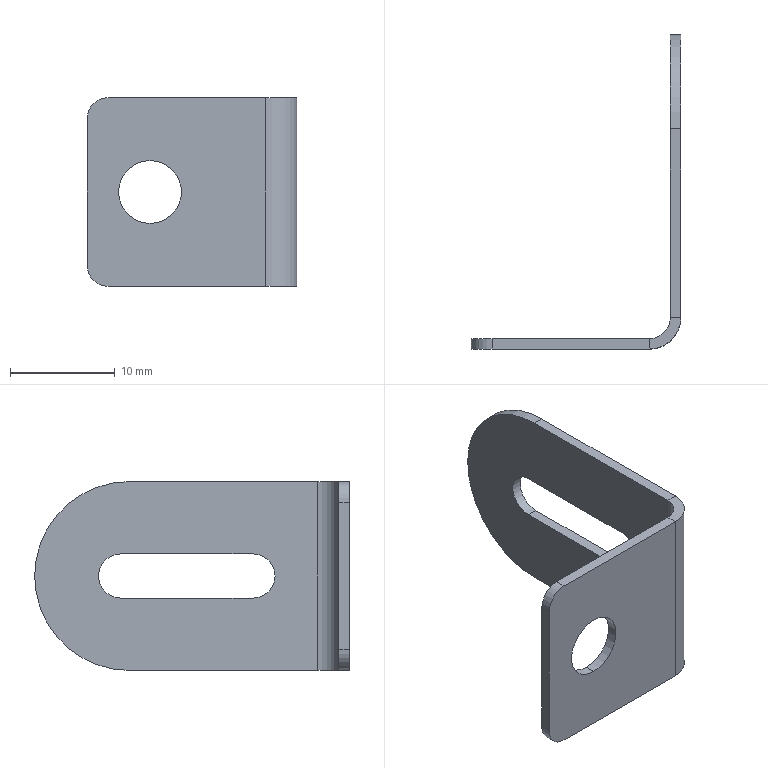Part | SolidWorks | features Fillet 2, ICE 2, EdgeFlange 1, FlatPattern 1, SMBaseFlange 1, SheetMetal 1 | 1 solid | 24 faces | box 20 x 30 x 18 mm | volume 730.964 mm3 | plane 13 | cylinder 11 | commonest cylinder face diameters 4 x3 4.2 x3 6 x3 18 x2
STEP:
#1=CARTESIAN_POINT('',(10.,8.173,2.1));
#2=VERTEX_POINT('',#1);
#3=CARTESIAN_POINT('',(10.,6.073,0.));
#4=VERTEX_POINT('',#3);
#5=CARTESIAN_POINT('',(10.,8.173,0.));
#6=DIRECTION('',(1.,0.,0.));
#7=DIRECTION('',(0.,1.,0.));
#8=AXIS2_PLACEMENT_3D('',#5,#6,#7);
#9=CIRCLE('',#8,2.1);
#10=EDGE_CURVE('',#2,#4,#9,.T.);
#11=ORIENTED_EDGE('',*,*,#10,.T.);
#12=CARTESIAN_POINT('',(9.,6.073,0.));
#13=VERTEX_POINT('',#12);
#14=CARTESIAN_POINT('',(19.,6.073,0.));
#15=DIRECTION('',(-1.,0.,0.));
#16=VECTOR('',#15,1000.);
#17=LINE('',#14,#16);
#18=EDGE_CURVE('',#4,#13,#17,.T.);
#19=ORIENTED_EDGE('',*,*,#18,.T.);
#20=CARTESIAN_POINT('',(9.,8.173,2.1));
#21=VERTEX_POINT('',#20);
#22=CARTESIAN_POINT('',(9.,8.173,0.));
#23=DIRECTION('',(-1.,0.,0.));
#24=DIRECTION('',(0.,-1.,0.));
#25=AXIS2_PLACEMENT_3D('',#22,#23,#24);
#26=CIRCLE('',#25,2.1);
#27=EDGE_CURVE('',#13,#21,#26,.T.);
#28=ORIENTED_EDGE('',*,*,#27,.T.);
#29=CARTESIAN_POINT('',(19.,8.173,2.1));
#30=DIRECTION('',(-1.,0.,0.));
#31=VECTOR('',#30,1000.);
#32=LINE('',#29,#31);
#33=EDGE_CURVE('',#2,#21,#32,.T.);
#34=ORIENTED_EDGE('',*,*,#33,.F.);
#35=EDGE_LOOP('',(#11,#19,#28,#34));
#36=FACE_OUTER_BOUND('',#35,.T.);
#37=CARTESIAN_POINT('',(19.,8.173,0.));
#38=DIRECTION('',(-1.,0.,0.));
#39=DIRECTION('',(0.,-1.,0.));
#40=AXIS2_PLACEMENT_3D('',#37,#38,#39);
#41=CYLINDRICAL_SURFACE('',#40,2.1);
#42=ADVANCED_FACE('',(#36),#41,.F.);
#43=CARTESIAN_POINT('',(-4.,-1.,-3.));
#44=VERTEX_POINT('',#43);
#45=CARTESIAN_POINT('',(-4.,-1.,3.));
#46=VERTEX_POINT('',#45);
#47=CARTESIAN_POINT('',(-4.,-1.,0.));
#48=DIRECTION('',(0.,1.,0.));
#49=DIRECTION('',(0.,0.,1.));
#50=AXIS2_PLACEMENT_3D('',#47,#48,#49);
#51=CIRCLE('',#50,3.);
#52=EDGE_CURVE('',#44,#46,#51,.T.);
#53=ORIENTED_EDGE('',*,*,#52,.F.);
#54=CARTESIAN_POINT('',(-4.,0.,-3.));
#55=VERTEX_POINT('',#54);
#56=CARTESIAN_POINT('',(-4.,-10.,-3.));
#57=DIRECTION('',(0.,1.,0.));
#58=VECTOR('',#57,1000.);
#59=LINE('',#56,#58);
#60=EDGE_CURVE('',#44,#55,#59,.T.);
#61=ORIENTED_EDGE('',*,*,#60,.T.);
#62=CARTESIAN_POINT('',(-4.,0.,3.));
#63=VERTEX_POINT('',#62);
#64=CARTESIAN_POINT('',(-4.,0.,0.));
#65=DIRECTION('',(0.,1.,0.));
#66=DIRECTION('',(0.,0.,1.));
#67=AXIS2_PLACEMENT_3D('',#64,#65,#66);
#68=CIRCLE('',#67,3.);
#69=EDGE_CURVE('',#55,#63,#68,.T.);
#70=ORIENTED_EDGE('',*,*,#69,.T.);
#71=CARTESIAN_POINT('',(-4.,-10.,3.));
#72=DIRECTION('',(0.,1.,0.));
#73=VECTOR('',#72,1000.);
#74=LINE('',#71,#73);
#75=EDGE_CURVE('',#46,#63,#74,.T.);
#76=ORIENTED_EDGE('',*,*,#75,.F.);
#77=EDGE_LOOP('',(#53,#61,#70,#76));
#78=FACE_OUTER_BOUND('',#77,.T.);
#79=CARTESIAN_POINT('',(-4.,-10.,0.));
#80=DIRECTION('',(0.,1.,0.));
#81=DIRECTION('',(0.,0.,1.));
#82=AXIS2_PLACEMENT_3D('',#79,#80,#81);
#83=CYLINDRICAL_SURFACE('',#82,3.);
#84=ADVANCED_FACE('',(#78),#83,.F.);
#85=CARTESIAN_POINT('',(7.,-1.,-9.));
#86=VERTEX_POINT('',#85);
#87=CARTESIAN_POINT('',(-8.,-1.,-9.));
#88=VERTEX_POINT('',#87);
#89=CARTESIAN_POINT('',(-10.,-1.,-9.));
#90=DIRECTION('',(-1.,0.,0.));
#91=VECTOR('',#90,1000.);
#92=LINE('',#89,#91);
#93=EDGE_CURVE('',#86,#88,#92,.T.);
#94=ORIENTED_EDGE('',*,*,#93,.T.);
#95=CARTESIAN_POINT('',(-8.,0.,-9.));
#96=VERTEX_POINT('',#95);
#97=CARTESIAN_POINT('',(-8.,-1.,-9.));
#98=DIRECTION('',(0.,1.,0.));
#99=VECTOR('',#98,1000.);
#100=LINE('',#97,#99);
#101=EDGE_CURVE('',#88,#96,#100,.T.);
#102=ORIENTED_EDGE('',*,*,#101,.T.);
#103=CARTESIAN_POINT('',(7.,0.,-9.));
#104=VERTEX_POINT('',#103);
#105=CARTESIAN_POINT('',(-10.,0.,-9.));
#106=DIRECTION('',(-1.,0.,0.));
#107=VECTOR('',#106,1000.);
#108=LINE('',#105,#107);
#109=EDGE_CURVE('',#104,#96,#108,.T.);
#110=ORIENTED_EDGE('',*,*,#109,.F.);
#111=CARTESIAN_POINT('',(7.,0.,-9.));
#112=DIRECTION('',(0.,-1.,0.));
#113=VECTOR('',#112,1000.);
#114=LINE('',#111,#113);
#115=EDGE_CURVE('',#104,#86,#114,.T.);
#116=ORIENTED_EDGE('',*,*,#115,.T.);
#117=EDGE_LOOP('',(#94,#102,#110,#116));
#118=FACE_OUTER_BOUND('',#117,.T.);
#119=CARTESIAN_POINT('',(-10.,-1.,-9.));
#120=DIRECTION('',(0.,0.,-1.));
#121=DIRECTION('',(-1.,0.,0.));
#122=AXIS2_PLACEMENT_3D('',#119,#120,#121);
#123=PLANE('',#122);
#124=ADVANCED_FACE('',(#118),#123,.T.);
#125=CARTESIAN_POINT('',(-4.,-1.,0.));
#126=DIRECTION('',(0.,1.,0.));
#127=DIRECTION('',(0.,0.,1.));
#128=AXIS2_PLACEMENT_3D('',#125,#126,#127);
#129=CIRCLE('',#128,3.);
#130=EDGE_CURVE('',#46,#44,#129,.T.);
#131=ORIENTED_EDGE('',*,*,#130,.T.);
#132=ORIENTED_EDGE('',*,*,#52,.T.);
#133=EDGE_LOOP('',(#131,#132));
#134=FACE_BOUND('',#133,.T.);
#135=CARTESIAN_POINT('',(-10.,-1.,-7.));
#136=VERTEX_POINT('',#135);
#137=CARTESIAN_POINT('',(-10.,-1.,7.));
#138=VERTEX_POINT('',#137);
#139=CARTESIAN_POINT('',(-10.,-1.,-9.));
#140=DIRECTION('',(0.,0.,1.));
#141=VECTOR('',#140,1000.);
#142=LINE('',#139,#141);
#143=EDGE_CURVE('',#136,#138,#142,.T.);
#144=ORIENTED_EDGE('',*,*,#143,.F.);
#145=CARTESIAN_POINT('',(-8.,-1.,-7.));
#146=DIRECTION('',(0.,-1.,0.));
#147=DIRECTION('',(0.,0.,1.));
#148=AXIS2_PLACEMENT_3D('',#145,#146,#147);
#149=CIRCLE('',#148,2.);
#150=EDGE_CURVE('',#136,#88,#149,.T.);
#151=ORIENTED_EDGE('',*,*,#150,.T.);
#152=ORIENTED_EDGE('',*,*,#93,.F.);
#153=CARTESIAN_POINT('',(7.,-1.,9.));
#154=VERTEX_POINT('',#153);
#155=CARTESIAN_POINT('',(7.,-1.,-9.));
#156=DIRECTION('',(0.,0.,1.));
#157=VECTOR('',#156,1000.);
#158=LINE('',#155,#157);
#159=EDGE_CURVE('',#86,#154,#158,.T.);
#160=ORIENTED_EDGE('',*,*,#159,.T.);
#161=CARTESIAN_POINT('',(-8.,-1.,9.));
#162=VERTEX_POINT('',#161);
#163=CARTESIAN_POINT('',(-10.,-1.,9.));
#164=DIRECTION('',(1.,0.,0.));
#165=VECTOR('',#164,1000.);
#166=LINE('',#163,#165);
#167=EDGE_CURVE('',#162,#154,#166,.T.);
#168=ORIENTED_EDGE('',*,*,#167,.F.);
#169=CARTESIAN_POINT('',(-8.,-1.,7.));
#170=DIRECTION('',(0.,-1.,0.));
#171=DIRECTION('',(0.,0.,1.));
#172=AXIS2_PLACEMENT_3D('',#169,#170,#171);
#173=CIRCLE('',#172,2.);
#174=EDGE_CURVE('',#162,#138,#173,.T.);
#175=ORIENTED_EDGE('',*,*,#174,.T.);
#176=EDGE_LOOP('',(#144,#151,#152,#160,#168,#175));
#177=FACE_OUTER_BOUND('',#176,.T.);
#178=CARTESIAN_POINT('',(0.,-1.,0.));
#179=DIRECTION('',(0.,1.,0.));
#180=DIRECTION('',(0.,0.,1.));
#181=AXIS2_PLACEMENT_3D('',#178,#179,#180);
#182=PLANE('',#181);
#183=ADVANCED_FACE('',(#134,#177),#182,.F.);
#184=CARTESIAN_POINT('',(-4.,0.,0.));
#185=DIRECTION('',(0.,1.,0.));
#186=DIRECTION('',(0.,0.,1.));
#187=AXIS2_PLACEMENT_3D('',#184,#185,#186);
#188=CIRCLE('',#187,3.);
#189=EDGE_CURVE('',#63,#55,#188,.T.);
#190=ORIENTED_EDGE('',*,*,#189,.F.);
#191=ORIENTED_EDGE('',*,*,#69,.F.);
#192=EDGE_LOOP('',(#190,#191));
#193=FACE_BOUND('',#192,.T.);
#194=ORIENTED_EDGE('',*,*,#109,.T.);
#195=CARTESIAN_POINT('',(-10.,0.,-7.));
#196=VERTEX_POINT('',#195);
#197=CARTESIAN_POINT('',(-8.,0.,-7.));
#198=DIRECTION('',(0.,1.,0.));
#199=DIRECTION('',(0.,0.,1.));
#200=AXIS2_PLACEMENT_3D('',#197,#198,#199);
#201=CIRCLE('',#200,2.);
#202=EDGE_CURVE('',#96,#196,#201,.T.);
#203=ORIENTED_EDGE('',*,*,#202,.T.);
#204=CARTESIAN_POINT('',(-10.,0.,7.));
#205=VERTEX_POINT('',#204);
#206=CARTESIAN_POINT('',(-10.,0.,-9.));
#207=DIRECTION('',(0.,0.,1.));
#208=VECTOR('',#207,1000.);
#209=LINE('',#206,#208);
#210=EDGE_CURVE('',#196,#205,#209,.T.);
#211=ORIENTED_EDGE('',*,*,#210,.T.);
#212=CARTESIAN_POINT('',(-8.,0.,9.));
#213=VERTEX_POINT('',#212);
#214=CARTESIAN_POINT('',(-8.,0.,7.));
#215=DIRECTION('',(0.,1.,0.));
#216=DIRECTION('',(0.,0.,1.));
#217=AXIS2_PLACEMENT_3D('',#214,#215,#216);
#218=CIRCLE('',#217,2.);
#219=EDGE_CURVE('',#205,#213,#218,.T.);
#220=ORIENTED_EDGE('',*,*,#219,.T.);
#221=CARTESIAN_POINT('',(7.,0.,9.));
#222=VERTEX_POINT('',#221);
#223=CARTESIAN_POINT('',(-10.,0.,9.));
#224=DIRECTION('',(1.,0.,0.));
#225=VECTOR('',#224,1000.);
#226=LINE('',#223,#225);
#227=EDGE_CURVE('',#213,#222,#226,.T.);
#228=ORIENTED_EDGE('',*,*,#227,.T.);
#229=CARTESIAN_POINT('',(7.,0.,-9.));
#230=DIRECTION('',(0.,0.,1.));
#231=VECTOR('',#230,1000.);
#232=LINE('',#229,#231);
#233=EDGE_CURVE('',#104,#222,#232,.T.);
#234=ORIENTED_EDGE('',*,*,#233,.F.);
#235=EDGE_LOOP('',(#194,#203,#211,#220,#228,#234));
#236=FACE_OUTER_BOUND('',#235,.T.);
#237=CARTESIAN_POINT('',(0.,0.,0.));
#238=DIRECTION('',(0.,1.,0.));
#239=DIRECTION('',(0.,0.,1.));
#240=AXIS2_PLACEMENT_3D('',#237,#238,#239);
#241=PLANE('',#240);
#242=ADVANCED_FACE('',(#193,#236),#241,.T.);
#243=ORIENTED_EDGE('',*,*,#227,.F.);
#244=CARTESIAN_POINT('',(-8.,-1.,9.));
#245=DIRECTION('',(0.,-1.,0.));
#246=VECTOR('',#245,1000.);
#247=LINE('',#244,#246);
#248=EDGE_CURVE('',#213,#162,#247,.T.);
#249=ORIENTED_EDGE('',*,*,#248,.T.);
#250=ORIENTED_EDGE('',*,*,#167,.T.);
#251=CARTESIAN_POINT('',(7.,0.,9.));
#252=DIRECTION('',(0.,-1.,0.));
#253=VECTOR('',#252,1000.);
#254=LINE('',#251,#253);
#255=EDGE_CURVE('',#222,#154,#254,.T.);
#256=ORIENTED_EDGE('',*,*,#255,.F.);
#257=EDGE_LOOP('',(#243,#249,#250,#256));
#258=FACE_OUTER_BOUND('',#257,.T.);
#259=CARTESIAN_POINT('',(-10.,-1.,9.));
#260=DIRECTION('',(0.,0.,1.));
#261=DIRECTION('',(1.,0.,0.));
#262=AXIS2_PLACEMENT_3D('',#259,#260,#261);
#263=PLANE('',#262);
#264=ADVANCED_FACE('',(#258),#263,.T.);
#265=ORIENTED_EDGE('',*,*,#210,.F.);
#266=CARTESIAN_POINT('',(-10.,-1.,-7.));
#267=DIRECTION('',(0.,-1.,0.));
#268=VECTOR('',#267,1000.);
#269=LINE('',#266,#268);
#270=EDGE_CURVE('',#196,#136,#269,.T.);
#271=ORIENTED_EDGE('',*,*,#270,.T.);
#272=ORIENTED_EDGE('',*,*,#143,.T.);
#273=CARTESIAN_POINT('',(-10.,-1.,7.));
#274=DIRECTION('',(0.,1.,0.));
#275=VECTOR('',#274,1000.);
#276=LINE('',#273,#275);
#277=EDGE_CURVE('',#138,#205,#276,.T.);
#278=ORIENTED_EDGE('',*,*,#277,.T.);
#279=EDGE_LOOP('',(#265,#271,#272,#278));
#280=FACE_OUTER_BOUND('',#279,.T.);
#281=CARTESIAN_POINT('',(-10.,-1.,-9.));
#282=DIRECTION('',(-1.,0.,0.));
#283=DIRECTION('',(0.,0.,1.));
#284=AXIS2_PLACEMENT_3D('',#281,#282,#283);
#285=PLANE('',#284);
#286=ADVANCED_FACE('',(#280),#285,.T.);
#287=CARTESIAN_POINT('',(9.,2.,9.));
#288=VERTEX_POINT('',#287);
#289=CARTESIAN_POINT('',(10.,2.,9.));
#290=VERTEX_POINT('',#289);
#291=CARTESIAN_POINT('',(10.,2.,9.));
#292=DIRECTION('',(1.,0.,0.));
#293=VECTOR('',#292,1000.);
#294=LINE('',#291,#293);
#295=EDGE_CURVE('',#288,#290,#294,.T.);
#296=ORIENTED_EDGE('',*,*,#295,.F.);
#297=CARTESIAN_POINT('',(7.,2.,9.));
#298=DIRECTION('',(0.,0.,1.));
#299=DIRECTION('',(-1.,0.,0.));
#300=AXIS2_PLACEMENT_3D('',#297,#298,#299);
#301=CIRCLE('',#300,2.);
#302=EDGE_CURVE('',#222,#288,#301,.T.);
#303=ORIENTED_EDGE('',*,*,#302,.F.);
#304=ORIENTED_EDGE('',*,*,#255,.T.);
#305=CARTESIAN_POINT('',(7.,2.,9.));
#306=DIRECTION('',(0.,0.,1.));
#307=DIRECTION('',(-1.,0.,0.));
#308=AXIS2_PLACEMENT_3D('',#305,#306,#307);
#309=CIRCLE('',#308,3.);
#310=EDGE_CURVE('',#154,#290,#309,.T.);
#311=ORIENTED_EDGE('',*,*,#310,.T.);
#312=EDGE_LOOP('',(#296,#303,#304,#311));
#313=FACE_OUTER_BOUND('',#312,.T.);
#314=CARTESIAN_POINT('',(7.,2.,9.));
#315=DIRECTION('',(0.,0.,1.));
#316=DIRECTION('',(1.,0.,0.));
#317=AXIS2_PLACEMENT_3D('',#314,#315,#316);
#318=PLANE('',#317);
#319=ADVANCED_FACE('',(#313),#318,.T.);
#320=CARTESIAN_POINT('',(9.,2.,-9.));
#321=VERTEX_POINT('',#320);
#322=CARTESIAN_POINT('',(7.,2.,-9.));
#323=DIRECTION('',(0.,0.,-1.));
#324=DIRECTION('',(-1.,0.,0.));
#325=AXIS2_PLACEMENT_3D('',#322,#323,#324);
#326=CIRCLE('',#325,2.);
#327=EDGE_CURVE('',#321,#104,#326,.T.);
#328=ORIENTED_EDGE('',*,*,#327,.F.);
#329=CARTESIAN_POINT('',(10.,2.,-9.));
#330=VERTEX_POINT('',#329);
#331=CARTESIAN_POINT('',(9.,2.,-9.));
#332=DIRECTION('',(1.,0.,0.));
#333=VECTOR('',#332,1000.);
#334=LINE('',#331,#333);
#335=EDGE_CURVE('',#321,#330,#334,.T.);
#336=ORIENTED_EDGE('',*,*,#335,.T.);
#337=CARTESIAN_POINT('',(7.,2.,-9.));
#338=DIRECTION('',(0.,0.,-1.));
#339=DIRECTION('',(-1.,0.,0.));
#340=AXIS2_PLACEMENT_3D('',#337,#338,#339);
#341=CIRCLE('',#340,3.);
#342=EDGE_CURVE('',#330,#86,#341,.T.);
#343=ORIENTED_EDGE('',*,*,#342,.T.);
#344=ORIENTED_EDGE('',*,*,#115,.F.);
#345=EDGE_LOOP('',(#328,#336,#343,#344));
#346=FACE_OUTER_BOUND('',#345,.T.);
#347=CARTESIAN_POINT('',(7.,2.,-9.));
#348=DIRECTION('',(0.,0.,1.));
#349=DIRECTION('',(1.,0.,0.));
#350=AXIS2_PLACEMENT_3D('',#347,#348,#349);
#351=PLANE('',#350);
#352=ADVANCED_FACE('',(#346),#351,.F.);
#353=ORIENTED_EDGE('',*,*,#159,.F.);
#354=ORIENTED_EDGE('',*,*,#342,.F.);
#355=CARTESIAN_POINT('',(10.,2.,0.));
#356=DIRECTION('',(0.,0.,-1.));
#357=VECTOR('',#356,1000.);
#358=LINE('',#355,#357);
#359=EDGE_CURVE('',#290,#330,#358,.T.);
#360=ORIENTED_EDGE('',*,*,#359,.F.);
#361=ORIENTED_EDGE('',*,*,#310,.F.);
#362=EDGE_LOOP('',(#353,#354,#360,#361));
#363=FACE_OUTER_BOUND('',#362,.T.);
#364=CARTESIAN_POINT('',(7.,2.,-9.));
#365=DIRECTION('',(0.,0.,-1.));
#366=DIRECTION('',(1.,0.,0.));
#367=AXIS2_PLACEMENT_3D('',#364,#365,#366);
#368=CYLINDRICAL_SURFACE('',#367,3.);
#369=ADVANCED_FACE('',(#363),#368,.T.);
#370=ORIENTED_EDGE('',*,*,#233,.T.);
#371=ORIENTED_EDGE('',*,*,#302,.T.);
#372=CARTESIAN_POINT('',(9.,2.,9.));
#373=DIRECTION('',(0.,0.,-1.));
#374=VECTOR('',#373,1000.);
#375=LINE('',#372,#374);
#376=EDGE_CURVE('',#288,#321,#375,.T.);
#377=ORIENTED_EDGE('',*,*,#376,.T.);
#378=ORIENTED_EDGE('',*,*,#327,.T.);
#379=EDGE_LOOP('',(#370,#371,#377,#378));
#380=FACE_OUTER_BOUND('',#379,.T.);
#381=CARTESIAN_POINT('',(7.,2.,-9.));
#382=DIRECTION('',(0.,0.,-1.));
#383=DIRECTION('',(1.,0.,0.));
#384=AXIS2_PLACEMENT_3D('',#381,#382,#383);
#385=CYLINDRICAL_SURFACE('',#384,2.);
#386=ADVANCED_FACE('',(#380),#385,.F.);
#387=CARTESIAN_POINT('',(9.,20.,-9.));
#388=VERTEX_POINT('',#387);
#389=CARTESIAN_POINT('',(9.,0.,-9.));
#390=DIRECTION('',(0.,-1.,0.));
#391=VECTOR('',#390,1000.);
#392=LINE('',#389,#391);
#393=EDGE_CURVE('',#388,#321,#392,.T.);
#394=ORIENTED_EDGE('',*,*,#393,.F.);
#395=CARTESIAN_POINT('',(10.,20.,-9.));
#396=VERTEX_POINT('',#395);
#397=CARTESIAN_POINT('',(10.,20.,-9.));
#398=DIRECTION('',(1.,0.,0.));
#399=VECTOR('',#398,1000.);
#400=LINE('',#397,#399);
#401=EDGE_CURVE('',#388,#396,#400,.T.);
#402=ORIENTED_EDGE('',*,*,#401,.T.);
#403=CARTESIAN_POINT('',(10.,0.,-9.));
#404=DIRECTION('',(0.,-1.,0.));
#405=VECTOR('',#404,1000.);
#406=LINE('',#403,#405);
#407=EDGE_CURVE('',#396,#330,#406,.T.);
#408=ORIENTED_EDGE('',*,*,#407,.T.);
#409=ORIENTED_EDGE('',*,*,#335,.F.);
#410=EDGE_LOOP('',(#394,#402,#408,#409));
#411=FACE_OUTER_BOUND('',#410,.T.);
#412=CARTESIAN_POINT('',(10.,0.,-9.));
#413=DIRECTION('',(0.,0.,-1.));
#414=DIRECTION('',(0.,1.,0.));
#415=AXIS2_PLACEMENT_3D('',#412,#413,#414);
#416=PLANE('',#415);
#417=ADVANCED_FACE('',(#411),#416,.T.);
#418=CARTESIAN_POINT('',(10.,20.,9.));
#419=VERTEX_POINT('',#418);
#420=CARTESIAN_POINT('',(10.,29.,9.));
#421=DIRECTION('',(0.,1.,0.));
#422=VECTOR('',#421,1000.);
#423=LINE('',#420,#422);
#424=EDGE_CURVE('',#290,#419,#423,.T.);
#425=ORIENTED_EDGE('',*,*,#424,.T.);
#426=CARTESIAN_POINT('',(9.,20.,9.));
#427=VERTEX_POINT('',#426);
#428=CARTESIAN_POINT('',(10.,20.,9.));
#429=DIRECTION('',(-1.,0.,0.));
#430=VECTOR('',#429,1000.);
#431=LINE('',#428,#430);
#432=EDGE_CURVE('',#419,#427,#431,.T.);
#433=ORIENTED_EDGE('',*,*,#432,.T.);
#434=CARTESIAN_POINT('',(9.,0.,9.));
#435=DIRECTION('',(0.,1.,0.));
#436=VECTOR('',#435,1000.);
#437=LINE('',#434,#436);
#438=EDGE_CURVE('',#288,#427,#437,.T.);
#439=ORIENTED_EDGE('',*,*,#438,.F.);
#440=ORIENTED_EDGE('',*,*,#295,.T.);
#441=EDGE_LOOP('',(#425,#433,#439,#440));
#442=FACE_OUTER_BOUND('',#441,.T.);
#443=CARTESIAN_POINT('',(10.,29.,9.));
#444=DIRECTION('',(0.,0.,1.));
#445=DIRECTION('',(1.,0.,0.));
#446=AXIS2_PLACEMENT_3D('',#443,#444,#445);
#447=PLANE('',#446);
#448=ADVANCED_FACE('',(#442),#447,.T.);
#449=CARTESIAN_POINT('',(10.,20.819,-2.1));
#450=VERTEX_POINT('',#449);
#451=CARTESIAN_POINT('',(10.,20.819,2.1));
#452=VERTEX_POINT('',#451);
#453=CARTESIAN_POINT('',(10.,20.819,0.));
#454=DIRECTION('',(1.,0.,0.));
#455=DIRECTION('',(0.,1.,0.));
#456=AXIS2_PLACEMENT_3D('',#453,#454,#455);
#457=CIRCLE('',#456,2.1);
#458=EDGE_CURVE('',#450,#452,#457,.T.);
#459=ORIENTED_EDGE('',*,*,#458,.F.);
#460=CARTESIAN_POINT('',(10.,8.173,-2.1));
#461=VERTEX_POINT('',#460);
#462=CARTESIAN_POINT('',(10.,0.,-2.1));
#463=DIRECTION('',(0.,1.,0.));
#464=VECTOR('',#463,1000.);
#465=LINE('',#462,#464);
#466=EDGE_CURVE('',#461,#450,#465,.T.);
#467=ORIENTED_EDGE('',*,*,#466,.F.);
#468=CARTESIAN_POINT('',(10.,8.173,0.));
#469=DIRECTION('',(1.,0.,0.));
#470=DIRECTION('',(0.,1.,0.));
#471=AXIS2_PLACEMENT_3D('',#468,#469,#470);
#472=CIRCLE('',#471,2.1);
#473=EDGE_CURVE('',#4,#461,#472,.T.);
#474=ORIENTED_EDGE('',*,*,#473,.F.);
#475=ORIENTED_EDGE('',*,*,#10,.F.);
#476=CARTESIAN_POINT('',(10.,0.,2.1));
#477=DIRECTION('',(0.,-1.,0.));
#478=VECTOR('',#477,1000.);
#479=LINE('',#476,#478);
#480=EDGE_CURVE('',#452,#2,#479,.T.);
#481=ORIENTED_EDGE('',*,*,#480,.F.);
#482=EDGE_LOOP('',(#459,#467,#474,#475,#481));
#483=FACE_BOUND('',#482,.T.);
#484=ORIENTED_EDGE('',*,*,#407,.F.);
#485=CARTESIAN_POINT('',(10.,29.,0.));
#486=VERTEX_POINT('',#485);
#487=CARTESIAN_POINT('',(10.,20.,0.));
#488=DIRECTION('',(1.,0.,0.));
#489=DIRECTION('',(0.,1.,0.));
#490=AXIS2_PLACEMENT_3D('',#487,#488,#489);
#491=CIRCLE('',#490,9.);
#492=EDGE_CURVE('',#396,#486,#491,.T.);
#493=ORIENTED_EDGE('',*,*,#492,.T.);
#494=CARTESIAN_POINT('',(10.,20.,0.));
#495=DIRECTION('',(1.,0.,0.));
#496=DIRECTION('',(0.,1.,0.));
#497=AXIS2_PLACEMENT_3D('',#494,#495,#496);
#498=CIRCLE('',#497,9.);
#499=EDGE_CURVE('',#486,#419,#498,.T.);
#500=ORIENTED_EDGE('',*,*,#499,.T.);
#501=ORIENTED_EDGE('',*,*,#424,.F.);
#502=ORIENTED_EDGE('',*,*,#359,.T.);
#503=EDGE_LOOP('',(#484,#493,#500,#501,#502));
#504=FACE_OUTER_BOUND('',#503,.T.);
#505=CARTESIAN_POINT('',(10.,0.,0.));
#506=DIRECTION('',(1.,0.,0.));
#507=DIRECTION('',(0.,1.,0.));
#508=AXIS2_PLACEMENT_3D('',#505,#506,#507);
#509=PLANE('',#508);
#510=ADVANCED_FACE('',(#483,#504),#509,.T.);
#511=CARTESIAN_POINT('',(9.,20.819,-2.1));
#512=VERTEX_POINT('',#511);
#513=CARTESIAN_POINT('',(9.,8.173,-2.1));
#514=VERTEX_POINT('',#513);
#515=CARTESIAN_POINT('',(9.,20.819,-2.1));
#516=DIRECTION('',(0.,-1.,0.));
#517=VECTOR('',#516,1000.);
#518=LINE('',#515,#517);
#519=EDGE_CURVE('',#512,#514,#518,.T.);
#520=ORIENTED_EDGE('',*,*,#519,.F.);
#521=CARTESIAN_POINT('',(9.,20.819,2.1));
#522=VERTEX_POINT('',#521);
#523=CARTESIAN_POINT('',(9.,20.819,0.));
#524=DIRECTION('',(-1.,0.,0.));
#525=DIRECTION('',(0.,-1.,0.));
#526=AXIS2_PLACEMENT_3D('',#523,#524,#525);
#527=CIRCLE('',#526,2.1);
#528=EDGE_CURVE('',#522,#512,#527,.T.);
#529=ORIENTED_EDGE('',*,*,#528,.F.);
#530=CARTESIAN_POINT('',(9.,20.819,2.1));
#531=DIRECTION('',(0.,1.,0.));
#532=VECTOR('',#531,1000.);
#533=LINE('',#530,#532);
#534=EDGE_CURVE('',#21,#522,#533,.T.);
#535=ORIENTED_EDGE('',*,*,#534,.F.);
#536=ORIENTED_EDGE('',*,*,#27,.F.);
#537=CARTESIAN_POINT('',(9.,8.173,0.));
#538=DIRECTION('',(-1.,0.,0.));
#539=DIRECTION('',(0.,-1.,0.));
#540=AXIS2_PLACEMENT_3D('',#537,#538,#539);
#541=CIRCLE('',#540,2.1);
#542=EDGE_CURVE('',#514,#13,#541,.T.);
#543=ORIENTED_EDGE('',*,*,#542,.F.);
#544=EDGE_LOOP('',(#520,#529,#535,#536,#543));
#545=FACE_BOUND('',#544,.T.);
#546=CARTESIAN_POINT('',(9.,29.,0.));
#547=VERTEX_POINT('',#546);
#548=CARTESIAN_POINT('',(9.,20.,0.));
#549=DIRECTION('',(-1.,0.,0.));
#550=DIRECTION('',(0.,1.,0.));
#551=AXIS2_PLACEMENT_3D('',#548,#549,#550);
#552=CIRCLE('',#551,9.);
#553=EDGE_CURVE('',#427,#547,#552,.T.);
#554=ORIENTED_EDGE('',*,*,#553,.T.);
#555=CARTESIAN_POINT('',(9.,20.,0.));
#556=DIRECTION('',(-1.,0.,0.));
#557=DIRECTION('',(0.,1.,0.));
#558=AXIS2_PLACEMENT_3D('',#555,#556,#557);
#559=CIRCLE('',#558,9.);
#560=EDGE_CURVE('',#547,#388,#559,.T.);
#561=ORIENTED_EDGE('',*,*,#560,.T.);
#562=ORIENTED_EDGE('',*,*,#393,.T.);
#563=ORIENTED_EDGE('',*,*,#376,.F.);
#564=ORIENTED_EDGE('',*,*,#438,.T.);
#565=EDGE_LOOP('',(#554,#561,#562,#563,#564));
#566=FACE_OUTER_BOUND('',#565,.T.);
#567=CARTESIAN_POINT('',(9.,0.,0.));
#568=DIRECTION('',(1.,0.,0.));
#569=DIRECTION('',(0.,1.,0.));
#570=AXIS2_PLACEMENT_3D('',#567,#568,#569);
#571=PLANE('',#570);
#572=ADVANCED_FACE('',(#545,#566),#571,.F.);
#573=ORIENTED_EDGE('',*,*,#60,.F.);
#574=ORIENTED_EDGE('',*,*,#130,.F.);
#575=ORIENTED_EDGE('',*,*,#75,.T.);
#576=ORIENTED_EDGE('',*,*,#189,.T.);
#577=EDGE_LOOP('',(#573,#574,#575,#576));
#578=FACE_OUTER_BOUND('',#577,.T.);
#579=CARTESIAN_POINT('',(-4.,-10.,0.));
#580=DIRECTION('',(0.,1.,0.));
#581=DIRECTION('',(0.,0.,1.));
#582=AXIS2_PLACEMENT_3D('',#579,#580,#581);
#583=CYLINDRICAL_SURFACE('',#582,3.);
#584=ADVANCED_FACE('',(#578),#583,.F.);
#585=ORIENTED_EDGE('',*,*,#432,.F.);
#586=ORIENTED_EDGE('',*,*,#499,.F.);
#587=CARTESIAN_POINT('',(10.,29.,0.));
#588=DIRECTION('',(1.,0.,0.));
#589=VECTOR('',#588,1000.);
#590=LINE('',#587,#589);
#591=EDGE_CURVE('',#547,#486,#590,.T.);
#592=ORIENTED_EDGE('',*,*,#591,.F.);
#593=ORIENTED_EDGE('',*,*,#553,.F.);
#594=EDGE_LOOP('',(#585,#586,#592,#593));
#595=FACE_OUTER_BOUND('',#594,.T.);
#596=CARTESIAN_POINT('',(10.,20.,0.));
#597=DIRECTION('',(-1.,0.,0.));
#598=DIRECTION('',(0.,-1.,0.));
#599=AXIS2_PLACEMENT_3D('',#596,#597,#598);
#600=CYLINDRICAL_SURFACE('',#599,9.);
#601=ADVANCED_FACE('',(#595),#600,.T.);
#602=ORIENTED_EDGE('',*,*,#492,.F.);
#603=ORIENTED_EDGE('',*,*,#401,.F.);
#604=ORIENTED_EDGE('',*,*,#560,.F.);
#605=ORIENTED_EDGE('',*,*,#591,.T.);
#606=EDGE_LOOP('',(#602,#603,#604,#605));
#607=FACE_OUTER_BOUND('',#606,.T.);
#608=CARTESIAN_POINT('',(10.,20.,0.));
#609=DIRECTION('',(-1.,0.,0.));
#610=DIRECTION('',(0.,-1.,0.));
#611=AXIS2_PLACEMENT_3D('',#608,#609,#610);
#612=CYLINDRICAL_SURFACE('',#611,9.);
#613=ADVANCED_FACE('',(#607),#612,.T.);
#614=ORIENTED_EDGE('',*,*,#458,.T.);
#615=CARTESIAN_POINT('',(19.,20.819,2.1));
#616=DIRECTION('',(-1.,0.,0.));
#617=VECTOR('',#616,1000.);
#618=LINE('',#615,#617);
#619=EDGE_CURVE('',#452,#522,#618,.T.);
#620=ORIENTED_EDGE('',*,*,#619,.T.);
#621=ORIENTED_EDGE('',*,*,#528,.T.);
#622=CARTESIAN_POINT('',(19.,20.819,-2.1));
#623=DIRECTION('',(-1.,0.,0.));
#624=VECTOR('',#623,1000.);
#625=LINE('',#622,#624);
#626=EDGE_CURVE('',#450,#512,#625,.T.);
#627=ORIENTED_EDGE('',*,*,#626,.F.);
#628=EDGE_LOOP('',(#614,#620,#621,#627));
#629=FACE_OUTER_BOUND('',#628,.T.);
#630=CARTESIAN_POINT('',(19.,20.819,0.));
#631=DIRECTION('',(-1.,0.,0.));
#632=DIRECTION('',(0.,-1.,0.));
#633=AXIS2_PLACEMENT_3D('',#630,#631,#632);
#634=CYLINDRICAL_SURFACE('',#633,2.1);
#635=ADVANCED_FACE('',(#629),#634,.F.);
#636=ORIENTED_EDGE('',*,*,#480,.T.);
#637=ORIENTED_EDGE('',*,*,#33,.T.);
#638=ORIENTED_EDGE('',*,*,#534,.T.);
#639=ORIENTED_EDGE('',*,*,#619,.F.);
#640=EDGE_LOOP('',(#636,#637,#638,#639));
#641=FACE_OUTER_BOUND('',#640,.T.);
#642=CARTESIAN_POINT('',(19.,20.819,2.1));
#643=DIRECTION('',(0.,0.,1.));
#644=DIRECTION('',(1.,0.,0.));
#645=AXIS2_PLACEMENT_3D('',#642,#643,#644);
#646=PLANE('',#645);
#647=ADVANCED_FACE('',(#641),#646,.F.);
#648=ORIENTED_EDGE('',*,*,#18,.F.);
#649=ORIENTED_EDGE('',*,*,#473,.T.);
#650=CARTESIAN_POINT('',(19.,8.173,-2.1));
#651=DIRECTION('',(-1.,0.,0.));
#652=VECTOR('',#651,1000.);
#653=LINE('',#650,#652);
#654=EDGE_CURVE('',#461,#514,#653,.T.);
#655=ORIENTED_EDGE('',*,*,#654,.T.);
#656=ORIENTED_EDGE('',*,*,#542,.T.);
#657=EDGE_LOOP('',(#648,#649,#655,#656));
#658=FACE_OUTER_BOUND('',#657,.T.);
#659=CARTESIAN_POINT('',(19.,8.173,0.));
#660=DIRECTION('',(-1.,0.,0.));
#661=DIRECTION('',(0.,-1.,0.));
#662=AXIS2_PLACEMENT_3D('',#659,#660,#661);
#663=CYLINDRICAL_SURFACE('',#662,2.1);
#664=ADVANCED_FACE('',(#658),#663,.F.);
#665=ORIENTED_EDGE('',*,*,#466,.T.);
#666=ORIENTED_EDGE('',*,*,#626,.T.);
#667=ORIENTED_EDGE('',*,*,#519,.T.);
#668=ORIENTED_EDGE('',*,*,#654,.F.);
#669=EDGE_LOOP('',(#665,#666,#667,#668));
#670=FACE_OUTER_BOUND('',#669,.T.);
#671=CARTESIAN_POINT('',(19.,20.819,-2.1));
#672=DIRECTION('',(0.,0.,-1.));
#673=DIRECTION('',(-1.,0.,0.));
#674=AXIS2_PLACEMENT_3D('',#671,#672,#673);
#675=PLANE('',#674);
#676=ADVANCED_FACE('',(#670),#675,.F.);
#677=ORIENTED_EDGE('',*,*,#150,.F.);
#678=ORIENTED_EDGE('',*,*,#270,.F.);
#679=ORIENTED_EDGE('',*,*,#202,.F.);
#680=ORIENTED_EDGE('',*,*,#101,.F.);
#681=EDGE_LOOP('',(#677,#678,#679,#680));
#682=FACE_OUTER_BOUND('',#681,.T.);
#683=CARTESIAN_POINT('',(-8.,-1.,-7.));
#684=DIRECTION('',(0.,1.,0.));
#685=DIRECTION('',(0.,0.,1.));
#686=AXIS2_PLACEMENT_3D('',#683,#684,#685);
#687=CYLINDRICAL_SURFACE('',#686,2.);
#688=ADVANCED_FACE('',(#682),#687,.T.);
#689=ORIENTED_EDGE('',*,*,#174,.F.);
#690=ORIENTED_EDGE('',*,*,#248,.F.);
#691=ORIENTED_EDGE('',*,*,#219,.F.);
#692=ORIENTED_EDGE('',*,*,#277,.F.);
#693=EDGE_LOOP('',(#689,#690,#691,#692));
#694=FACE_OUTER_BOUND('',#693,.T.);
#695=CARTESIAN_POINT('',(-8.,-1.,7.));
#696=DIRECTION('',(0.,1.,0.));
#697=DIRECTION('',(0.,0.,1.));
#698=AXIS2_PLACEMENT_3D('',#695,#696,#697);
#699=CYLINDRICAL_SURFACE('',#698,2.);
#700=ADVANCED_FACE('',(#694),#699,.T.);
#701=CLOSED_SHELL('',(#42,#84,#124,#183,#242,#264,#286,#319,#352,#369,#386,#417,#448,#510,#572,#584,#601,#613,#635,#647,#664,#676,#688,#700));
#702=MANIFOLD_SOLID_BREP('',#701);
#703=CARTESIAN_POINT('',(0.,0.,0.));
#704=DIRECTION('',(0.,0.,1.));
#705=DIRECTION('',(1.,0.,0.));
#706=AXIS2_PLACEMENT_3D('',#703,#704,#705);
#707=(LENGTH_UNIT()NAMED_UNIT(*)SI_UNIT(.MILLI.,.METRE.));
#708=UNCERTAINTY_MEASURE_WITH_UNIT(LENGTH_MEASURE(0.00001),#707,'','');
#709=(NAMED_UNIT(*)PLANE_ANGLE_UNIT()SI_UNIT($,.RADIAN.));
#710=(NAMED_UNIT(*)SI_UNIT($,.STERADIAN.)SOLID_ANGLE_UNIT());
#711=(GEOMETRIC_REPRESENTATION_CONTEXT(3)GLOBAL_UNCERTAINTY_ASSIGNED_CONTEXT((#708))GLOBAL_UNIT_ASSIGNED_CONTEXT((#707,#709,#710))REPRESENTATION_CONTEXT('',''));
#712=ADVANCED_BREP_SHAPE_REPRESENTATION('',(#702,#706),#711);